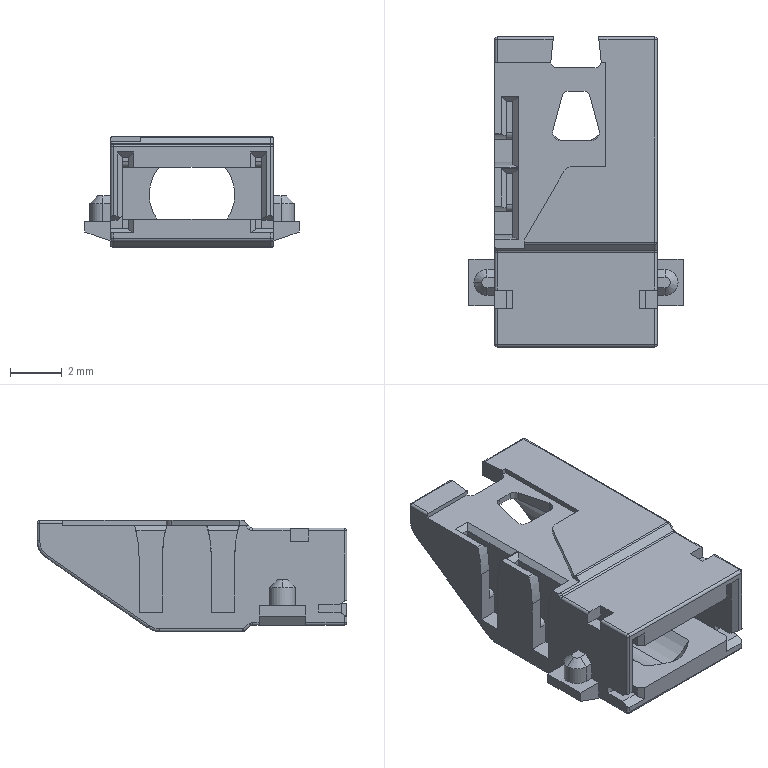Part | Creo | 1 solid | 220 faces | box 8.3 x 12 x 4.3 mm | volume 132.29 mm3 | plane 132 | cylinder 59 | cone 9 | sphere 9 | torus 7 | other 4 | commonest cylinder face diameters 0.2 x33 0.5 x11 0.6 x3 1 x3 1.6 x3 3.1 x3